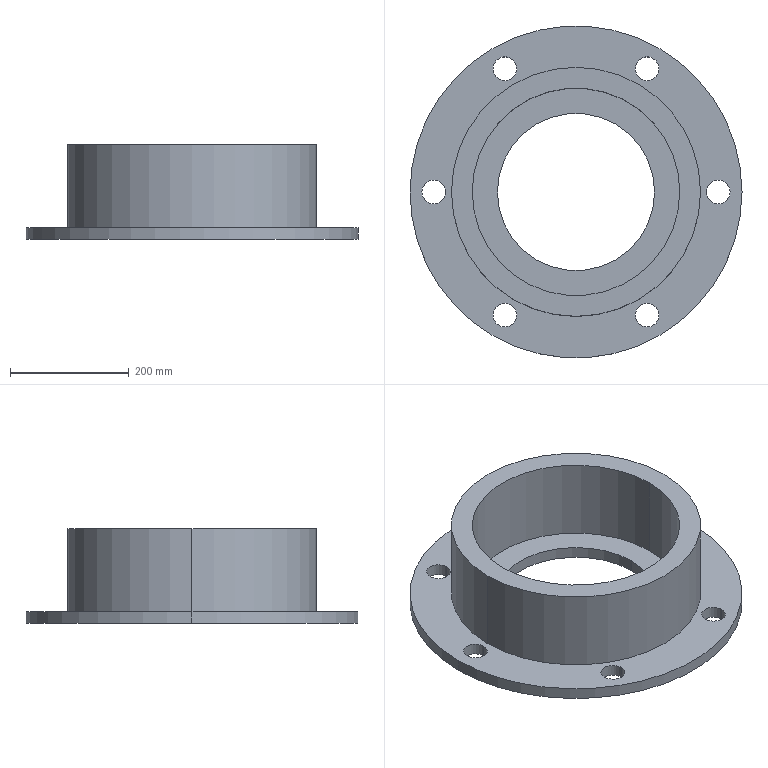Part | SolidWorks | features ICE 4, 3DProfileFeature 1, Extrusion 1 | 1 solid | 24 faces | box 560 x 560 x 160 mm | volume 9598744 mm3 | cylinder 20 | plane 4 | commonest cylinder face diameters 40 x12 265 x2 350 x2 420 x2 560 x2
STEP:
#1=CARTESIAN_POINT('',(-132.5,0.,20.));
#2=VERTEX_POINT('',#1);
#3=CARTESIAN_POINT('',(132.5,0.,20.));
#4=VERTEX_POINT('',#3);
#5=CARTESIAN_POINT('',(0.,0.,20.));
#6=DIRECTION('',(0.,0.,1.));
#7=DIRECTION('',(1.,0.,0.));
#8=AXIS2_PLACEMENT_3D('',#5,#6,#7);
#9=CIRCLE('',#8,132.5);
#10=EDGE_CURVE('',#2,#4,#9,.T.);
#11=ORIENTED_EDGE('',*,*,#10,.T.);
#12=CARTESIAN_POINT('',(132.5,0.,0.));
#13=VERTEX_POINT('',#12);
#14=CARTESIAN_POINT('',(132.5,0.,20.));
#15=DIRECTION('',(0.,0.,-1.));
#16=VECTOR('',#15,1000.);
#17=LINE('',#14,#16);
#18=EDGE_CURVE('',#4,#13,#17,.T.);
#19=ORIENTED_EDGE('',*,*,#18,.T.);
#20=CARTESIAN_POINT('',(-132.5,0.,0.));
#21=VERTEX_POINT('',#20);
#22=CARTESIAN_POINT('',(0.,0.,0.));
#23=DIRECTION('',(0.,0.,1.));
#24=DIRECTION('',(1.,0.,0.));
#25=AXIS2_PLACEMENT_3D('',#22,#23,#24);
#26=CIRCLE('',#25,132.5);
#27=EDGE_CURVE('',#21,#13,#26,.T.);
#28=ORIENTED_EDGE('',*,*,#27,.F.);
#29=CARTESIAN_POINT('',(-132.5,0.,20.));
#30=DIRECTION('',(0.,0.,-1.));
#31=VECTOR('',#30,1000.);
#32=LINE('',#29,#31);
#33=EDGE_CURVE('',#2,#21,#32,.T.);
#34=ORIENTED_EDGE('',*,*,#33,.F.);
#35=EDGE_LOOP('',(#11,#19,#28,#34));
#36=FACE_OUTER_BOUND('',#35,.T.);
#37=CARTESIAN_POINT('',(0.,0.,20.));
#38=DIRECTION('',(0.,0.,-1.));
#39=DIRECTION('',(-1.,0.,0.));
#40=AXIS2_PLACEMENT_3D('',#37,#38,#39);
#41=CYLINDRICAL_SURFACE('',#40,132.5);
#42=ADVANCED_FACE('',(#36),#41,.F.);
#43=CARTESIAN_POINT('',(220.,0.,20.));
#44=VERTEX_POINT('',#43);
#45=CARTESIAN_POINT('',(260.,0.,20.));
#46=VERTEX_POINT('',#45);
#47=CARTESIAN_POINT('',(240.,0.,20.));
#48=DIRECTION('',(0.,0.,1.));
#49=DIRECTION('',(1.,0.,0.));
#50=AXIS2_PLACEMENT_3D('',#47,#48,#49);
#51=CIRCLE('',#50,20.);
#52=EDGE_CURVE('',#44,#46,#51,.T.);
#53=ORIENTED_EDGE('',*,*,#52,.T.);
#54=CARTESIAN_POINT('',(260.,0.,0.));
#55=VERTEX_POINT('',#54);
#56=CARTESIAN_POINT('',(260.,0.,20.));
#57=DIRECTION('',(0.,0.,-1.));
#58=VECTOR('',#57,1000.);
#59=LINE('',#56,#58);
#60=EDGE_CURVE('',#46,#55,#59,.T.);
#61=ORIENTED_EDGE('',*,*,#60,.T.);
#62=CARTESIAN_POINT('',(220.,0.,0.));
#63=VERTEX_POINT('',#62);
#64=CARTESIAN_POINT('',(240.,0.,0.));
#65=DIRECTION('',(0.,0.,1.));
#66=DIRECTION('',(1.,0.,0.));
#67=AXIS2_PLACEMENT_3D('',#64,#65,#66);
#68=CIRCLE('',#67,20.);
#69=EDGE_CURVE('',#63,#55,#68,.T.);
#70=ORIENTED_EDGE('',*,*,#69,.F.);
#71=CARTESIAN_POINT('',(220.,0.,20.));
#72=DIRECTION('',(0.,0.,-1.));
#73=VECTOR('',#72,1000.);
#74=LINE('',#71,#73);
#75=EDGE_CURVE('',#44,#63,#74,.T.);
#76=ORIENTED_EDGE('',*,*,#75,.F.);
#77=EDGE_LOOP('',(#53,#61,#70,#76));
#78=FACE_OUTER_BOUND('',#77,.T.);
#79=CARTESIAN_POINT('',(240.,0.,20.));
#80=DIRECTION('',(0.,0.,-1.));
#81=DIRECTION('',(-1.,0.,0.));
#82=AXIS2_PLACEMENT_3D('',#79,#80,#81);
#83=CYLINDRICAL_SURFACE('',#82,20.);
#84=ADVANCED_FACE('',(#78),#83,.F.);
#85=CARTESIAN_POINT('',(100.,-207.846,20.));
#86=VERTEX_POINT('',#85);
#87=CARTESIAN_POINT('',(140.,-207.846,20.));
#88=VERTEX_POINT('',#87);
#89=CARTESIAN_POINT('',(120.,-207.846,20.));
#90=DIRECTION('',(0.,0.,1.));
#91=DIRECTION('',(1.,0.,0.));
#92=AXIS2_PLACEMENT_3D('',#89,#90,#91);
#93=CIRCLE('',#92,20.);
#94=EDGE_CURVE('',#86,#88,#93,.T.);
#95=ORIENTED_EDGE('',*,*,#94,.T.);
#96=CARTESIAN_POINT('',(140.,-207.846,0.));
#97=VERTEX_POINT('',#96);
#98=CARTESIAN_POINT('',(140.,-207.846,20.));
#99=DIRECTION('',(0.,0.,-1.));
#100=VECTOR('',#99,1000.);
#101=LINE('',#98,#100);
#102=EDGE_CURVE('',#88,#97,#101,.T.);
#103=ORIENTED_EDGE('',*,*,#102,.T.);
#104=CARTESIAN_POINT('',(100.,-207.846,0.));
#105=VERTEX_POINT('',#104);
#106=CARTESIAN_POINT('',(120.,-207.846,0.));
#107=DIRECTION('',(0.,0.,1.));
#108=DIRECTION('',(1.,0.,0.));
#109=AXIS2_PLACEMENT_3D('',#106,#107,#108);
#110=CIRCLE('',#109,20.);
#111=EDGE_CURVE('',#105,#97,#110,.T.);
#112=ORIENTED_EDGE('',*,*,#111,.F.);
#113=CARTESIAN_POINT('',(100.,-207.846,20.));
#114=DIRECTION('',(0.,0.,-1.));
#115=VECTOR('',#114,1000.);
#116=LINE('',#113,#115);
#117=EDGE_CURVE('',#86,#105,#116,.T.);
#118=ORIENTED_EDGE('',*,*,#117,.F.);
#119=EDGE_LOOP('',(#95,#103,#112,#118));
#120=FACE_OUTER_BOUND('',#119,.T.);
#121=CARTESIAN_POINT('',(120.,-207.846,20.));
#122=DIRECTION('',(0.,0.,-1.));
#123=DIRECTION('',(-1.,0.,0.));
#124=AXIS2_PLACEMENT_3D('',#121,#122,#123);
#125=CYLINDRICAL_SURFACE('',#124,20.);
#126=ADVANCED_FACE('',(#120),#125,.F.);
#127=CARTESIAN_POINT('',(-260.,0.,20.));
#128=VERTEX_POINT('',#127);
#129=CARTESIAN_POINT('',(-220.,0.,20.));
#130=VERTEX_POINT('',#129);
#131=CARTESIAN_POINT('',(-240.,0.,20.));
#132=DIRECTION('',(0.,0.,1.));
#133=DIRECTION('',(1.,0.,0.));
#134=AXIS2_PLACEMENT_3D('',#131,#132,#133);
#135=CIRCLE('',#134,20.);
#136=EDGE_CURVE('',#128,#130,#135,.T.);
#137=ORIENTED_EDGE('',*,*,#136,.T.);
#138=CARTESIAN_POINT('',(-220.,0.,0.));
#139=VERTEX_POINT('',#138);
#140=CARTESIAN_POINT('',(-220.,0.,20.));
#141=DIRECTION('',(0.,0.,-1.));
#142=VECTOR('',#141,1000.);
#143=LINE('',#140,#142);
#144=EDGE_CURVE('',#130,#139,#143,.T.);
#145=ORIENTED_EDGE('',*,*,#144,.T.);
#146=CARTESIAN_POINT('',(-260.,0.,0.));
#147=VERTEX_POINT('',#146);
#148=CARTESIAN_POINT('',(-240.,0.,0.));
#149=DIRECTION('',(0.,0.,1.));
#150=DIRECTION('',(1.,0.,0.));
#151=AXIS2_PLACEMENT_3D('',#148,#149,#150);
#152=CIRCLE('',#151,20.);
#153=EDGE_CURVE('',#147,#139,#152,.T.);
#154=ORIENTED_EDGE('',*,*,#153,.F.);
#155=CARTESIAN_POINT('',(-260.,0.,20.));
#156=DIRECTION('',(0.,0.,-1.));
#157=VECTOR('',#156,1000.);
#158=LINE('',#155,#157);
#159=EDGE_CURVE('',#128,#147,#158,.T.);
#160=ORIENTED_EDGE('',*,*,#159,.F.);
#161=EDGE_LOOP('',(#137,#145,#154,#160));
#162=FACE_OUTER_BOUND('',#161,.T.);
#163=CARTESIAN_POINT('',(-240.,0.,20.));
#164=DIRECTION('',(0.,0.,-1.));
#165=DIRECTION('',(-1.,0.,0.));
#166=AXIS2_PLACEMENT_3D('',#163,#164,#165);
#167=CYLINDRICAL_SURFACE('',#166,20.);
#168=ADVANCED_FACE('',(#162),#167,.F.);
#169=CARTESIAN_POINT('',(-140.,207.846,20.));
#170=VERTEX_POINT('',#169);
#171=CARTESIAN_POINT('',(-100.,207.846,20.));
#172=VERTEX_POINT('',#171);
#173=CARTESIAN_POINT('',(-120.,207.846,20.));
#174=DIRECTION('',(0.,0.,1.));
#175=DIRECTION('',(1.,0.,0.));
#176=AXIS2_PLACEMENT_3D('',#173,#174,#175);
#177=CIRCLE('',#176,20.);
#178=EDGE_CURVE('',#170,#172,#177,.T.);
#179=ORIENTED_EDGE('',*,*,#178,.T.);
#180=CARTESIAN_POINT('',(-100.,207.846,0.));
#181=VERTEX_POINT('',#180);
#182=CARTESIAN_POINT('',(-100.,207.846,20.));
#183=DIRECTION('',(0.,0.,-1.));
#184=VECTOR('',#183,1000.);
#185=LINE('',#182,#184);
#186=EDGE_CURVE('',#172,#181,#185,.T.);
#187=ORIENTED_EDGE('',*,*,#186,.T.);
#188=CARTESIAN_POINT('',(-140.,207.846,0.));
#189=VERTEX_POINT('',#188);
#190=CARTESIAN_POINT('',(-120.,207.846,0.));
#191=DIRECTION('',(0.,0.,1.));
#192=DIRECTION('',(1.,0.,0.));
#193=AXIS2_PLACEMENT_3D('',#190,#191,#192);
#194=CIRCLE('',#193,20.);
#195=EDGE_CURVE('',#189,#181,#194,.T.);
#196=ORIENTED_EDGE('',*,*,#195,.F.);
#197=CARTESIAN_POINT('',(-140.,207.846,20.));
#198=DIRECTION('',(0.,0.,-1.));
#199=VECTOR('',#198,1000.);
#200=LINE('',#197,#199);
#201=EDGE_CURVE('',#170,#189,#200,.T.);
#202=ORIENTED_EDGE('',*,*,#201,.F.);
#203=EDGE_LOOP('',(#179,#187,#196,#202));
#204=FACE_OUTER_BOUND('',#203,.T.);
#205=CARTESIAN_POINT('',(-120.,207.846,20.));
#206=DIRECTION('',(0.,0.,-1.));
#207=DIRECTION('',(-1.,0.,0.));
#208=AXIS2_PLACEMENT_3D('',#205,#206,#207);
#209=CYLINDRICAL_SURFACE('',#208,20.);
#210=ADVANCED_FACE('',(#204),#209,.F.);
#211=CARTESIAN_POINT('',(100.,207.846,20.));
#212=VERTEX_POINT('',#211);
#213=CARTESIAN_POINT('',(140.,207.846,20.));
#214=VERTEX_POINT('',#213);
#215=CARTESIAN_POINT('',(120.,207.846,20.));
#216=DIRECTION('',(0.,0.,1.));
#217=DIRECTION('',(1.,0.,0.));
#218=AXIS2_PLACEMENT_3D('',#215,#216,#217);
#219=CIRCLE('',#218,20.);
#220=EDGE_CURVE('',#212,#214,#219,.T.);
#221=ORIENTED_EDGE('',*,*,#220,.T.);
#222=CARTESIAN_POINT('',(140.,207.846,0.));
#223=VERTEX_POINT('',#222);
#224=CARTESIAN_POINT('',(140.,207.846,20.));
#225=DIRECTION('',(0.,0.,-1.));
#226=VECTOR('',#225,1000.);
#227=LINE('',#224,#226);
#228=EDGE_CURVE('',#214,#223,#227,.T.);
#229=ORIENTED_EDGE('',*,*,#228,.T.);
#230=CARTESIAN_POINT('',(100.,207.846,0.));
#231=VERTEX_POINT('',#230);
#232=CARTESIAN_POINT('',(120.,207.846,0.));
#233=DIRECTION('',(0.,0.,1.));
#234=DIRECTION('',(1.,0.,0.));
#235=AXIS2_PLACEMENT_3D('',#232,#233,#234);
#236=CIRCLE('',#235,20.);
#237=EDGE_CURVE('',#231,#223,#236,.T.);
#238=ORIENTED_EDGE('',*,*,#237,.F.);
#239=CARTESIAN_POINT('',(100.,207.846,20.));
#240=DIRECTION('',(0.,0.,-1.));
#241=VECTOR('',#240,1000.);
#242=LINE('',#239,#241);
#243=EDGE_CURVE('',#212,#231,#242,.T.);
#244=ORIENTED_EDGE('',*,*,#243,.F.);
#245=EDGE_LOOP('',(#221,#229,#238,#244));
#246=FACE_OUTER_BOUND('',#245,.T.);
#247=CARTESIAN_POINT('',(120.,207.846,20.));
#248=DIRECTION('',(0.,0.,-1.));
#249=DIRECTION('',(-1.,0.,0.));
#250=AXIS2_PLACEMENT_3D('',#247,#248,#249);
#251=CYLINDRICAL_SURFACE('',#250,20.);
#252=ADVANCED_FACE('',(#246),#251,.F.);
#253=CARTESIAN_POINT('',(-140.,-207.846,20.));
#254=VERTEX_POINT('',#253);
#255=CARTESIAN_POINT('',(-100.,-207.846,20.));
#256=VERTEX_POINT('',#255);
#257=CARTESIAN_POINT('',(-120.,-207.846,20.));
#258=DIRECTION('',(0.,0.,1.));
#259=DIRECTION('',(1.,0.,0.));
#260=AXIS2_PLACEMENT_3D('',#257,#258,#259);
#261=CIRCLE('',#260,20.);
#262=EDGE_CURVE('',#254,#256,#261,.T.);
#263=ORIENTED_EDGE('',*,*,#262,.T.);
#264=CARTESIAN_POINT('',(-100.,-207.846,0.));
#265=VERTEX_POINT('',#264);
#266=CARTESIAN_POINT('',(-100.,-207.846,20.));
#267=DIRECTION('',(0.,0.,-1.));
#268=VECTOR('',#267,1000.);
#269=LINE('',#266,#268);
#270=EDGE_CURVE('',#256,#265,#269,.T.);
#271=ORIENTED_EDGE('',*,*,#270,.T.);
#272=CARTESIAN_POINT('',(-140.,-207.846,0.));
#273=VERTEX_POINT('',#272);
#274=CARTESIAN_POINT('',(-120.,-207.846,0.));
#275=DIRECTION('',(0.,0.,1.));
#276=DIRECTION('',(1.,0.,0.));
#277=AXIS2_PLACEMENT_3D('',#274,#275,#276);
#278=CIRCLE('',#277,20.);
#279=EDGE_CURVE('',#273,#265,#278,.T.);
#280=ORIENTED_EDGE('',*,*,#279,.F.);
#281=CARTESIAN_POINT('',(-140.,-207.846,20.));
#282=DIRECTION('',(0.,0.,-1.));
#283=VECTOR('',#282,1000.);
#284=LINE('',#281,#283);
#285=EDGE_CURVE('',#254,#273,#284,.T.);
#286=ORIENTED_EDGE('',*,*,#285,.F.);
#287=EDGE_LOOP('',(#263,#271,#280,#286));
#288=FACE_OUTER_BOUND('',#287,.T.);
#289=CARTESIAN_POINT('',(-120.,-207.846,20.));
#290=DIRECTION('',(0.,0.,-1.));
#291=DIRECTION('',(-1.,0.,0.));
#292=AXIS2_PLACEMENT_3D('',#289,#290,#291);
#293=CYLINDRICAL_SURFACE('',#292,20.);
#294=ADVANCED_FACE('',(#288),#293,.F.);
#295=CARTESIAN_POINT('',(175.,0.,20.));
#296=VERTEX_POINT('',#295);
#297=CARTESIAN_POINT('',(-175.,0.,20.));
#298=VERTEX_POINT('',#297);
#299=CARTESIAN_POINT('',(0.,0.,20.));
#300=DIRECTION('',(0.,0.,-1.));
#301=DIRECTION('',(1.,0.,0.));
#302=AXIS2_PLACEMENT_3D('',#299,#300,#301);
#303=CIRCLE('',#302,175.);
#304=EDGE_CURVE('',#296,#298,#303,.T.);
#305=ORIENTED_EDGE('',*,*,#304,.T.);
#306=CARTESIAN_POINT('',(-175.,0.,160.));
#307=VERTEX_POINT('',#306);
#308=CARTESIAN_POINT('',(-175.,0.,-474.975));
#309=DIRECTION('',(0.,0.,1.));
#310=VECTOR('',#309,1000.);
#311=LINE('',#308,#310);
#312=EDGE_CURVE('',#298,#307,#311,.T.);
#313=ORIENTED_EDGE('',*,*,#312,.T.);
#314=CARTESIAN_POINT('',(175.,0.,160.));
#315=VERTEX_POINT('',#314);
#316=CARTESIAN_POINT('',(0.,0.,160.));
#317=DIRECTION('',(0.,0.,1.));
#318=DIRECTION('',(1.,0.,0.));
#319=AXIS2_PLACEMENT_3D('',#316,#317,#318);
#320=CIRCLE('',#319,175.);
#321=EDGE_CURVE('',#307,#315,#320,.T.);
#322=ORIENTED_EDGE('',*,*,#321,.T.);
#323=CARTESIAN_POINT('',(175.,0.,-474.975));
#324=DIRECTION('',(0.,0.,1.));
#325=VECTOR('',#324,1000.);
#326=LINE('',#323,#325);
#327=EDGE_CURVE('',#296,#315,#326,.T.);
#328=ORIENTED_EDGE('',*,*,#327,.F.);
#329=EDGE_LOOP('',(#305,#313,#322,#328));
#330=FACE_OUTER_BOUND('',#329,.T.);
#331=CARTESIAN_POINT('',(0.,0.,-474.975));
#332=DIRECTION('',(0.,0.,1.));
#333=DIRECTION('',(1.,0.,0.));
#334=AXIS2_PLACEMENT_3D('',#331,#332,#333);
#335=CYLINDRICAL_SURFACE('',#334,175.);
#336=ADVANCED_FACE('',(#330),#335,.F.);
#337=CARTESIAN_POINT('',(210.,0.,160.));
#338=VERTEX_POINT('',#337);
#339=CARTESIAN_POINT('',(-210.,0.,160.));
#340=VERTEX_POINT('',#339);
#341=CARTESIAN_POINT('',(0.,0.,160.));
#342=DIRECTION('',(0.,0.,1.));
#343=DIRECTION('',(1.,0.,0.));
#344=AXIS2_PLACEMENT_3D('',#341,#342,#343);
#345=CIRCLE('',#344,210.);
#346=EDGE_CURVE('',#338,#340,#345,.T.);
#347=ORIENTED_EDGE('',*,*,#346,.F.);
#348=CARTESIAN_POINT('',(210.,0.,20.));
#349=VERTEX_POINT('',#348);
#350=CARTESIAN_POINT('',(210.,0.,160.));
#351=DIRECTION('',(0.,0.,-1.));
#352=VECTOR('',#351,1000.);
#353=LINE('',#350,#352);
#354=EDGE_CURVE('',#338,#349,#353,.T.);
#355=ORIENTED_EDGE('',*,*,#354,.T.);
#356=CARTESIAN_POINT('',(-210.,0.,20.));
#357=VERTEX_POINT('',#356);
#358=CARTESIAN_POINT('',(0.,0.,20.));
#359=DIRECTION('',(0.,0.,-1.));
#360=DIRECTION('',(1.,0.,0.));
#361=AXIS2_PLACEMENT_3D('',#358,#359,#360);
#362=CIRCLE('',#361,210.);
#363=EDGE_CURVE('',#357,#349,#362,.T.);
#364=ORIENTED_EDGE('',*,*,#363,.F.);
#365=CARTESIAN_POINT('',(-210.,0.,160.));
#366=DIRECTION('',(0.,0.,-1.));
#367=VECTOR('',#366,1000.);
#368=LINE('',#365,#367);
#369=EDGE_CURVE('',#340,#357,#368,.T.);
#370=ORIENTED_EDGE('',*,*,#369,.F.);
#371=EDGE_LOOP('',(#347,#355,#364,#370));
#372=FACE_OUTER_BOUND('',#371,.T.);
#373=CARTESIAN_POINT('',(0.,0.,160.));
#374=DIRECTION('',(0.,0.,-1.));
#375=DIRECTION('',(-1.,0.,0.));
#376=AXIS2_PLACEMENT_3D('',#373,#374,#375);
#377=CYLINDRICAL_SURFACE('',#376,210.);
#378=ADVANCED_FACE('',(#372),#377,.T.);
#379=CARTESIAN_POINT('',(280.,0.,20.));
#380=VERTEX_POINT('',#379);
#381=CARTESIAN_POINT('',(-280.,0.,20.));
#382=VERTEX_POINT('',#381);
#383=CARTESIAN_POINT('',(0.,0.,20.));
#384=DIRECTION('',(0.,0.,1.));
#385=DIRECTION('',(1.,0.,0.));
#386=AXIS2_PLACEMENT_3D('',#383,#384,#385);
#387=CIRCLE('',#386,280.);
#388=EDGE_CURVE('',#380,#382,#387,.T.);
#389=ORIENTED_EDGE('',*,*,#388,.F.);
#390=CARTESIAN_POINT('',(280.,0.,0.));
#391=VERTEX_POINT('',#390);
#392=CARTESIAN_POINT('',(280.,0.,20.));
#393=DIRECTION('',(0.,0.,-1.));
#394=VECTOR('',#393,1000.);
#395=LINE('',#392,#394);
#396=EDGE_CURVE('',#380,#391,#395,.T.);
#397=ORIENTED_EDGE('',*,*,#396,.T.);
#398=CARTESIAN_POINT('',(-280.,0.,0.));
#399=VERTEX_POINT('',#398);
#400=CARTESIAN_POINT('',(0.,0.,0.));
#401=DIRECTION('',(0.,0.,1.));
#402=DIRECTION('',(1.,0.,0.));
#403=AXIS2_PLACEMENT_3D('',#400,#401,#402);
#404=CIRCLE('',#403,280.);
#405=EDGE_CURVE('',#391,#399,#404,.T.);
#406=ORIENTED_EDGE('',*,*,#405,.T.);
#407=CARTESIAN_POINT('',(-280.,0.,20.));
#408=DIRECTION('',(0.,0.,-1.));
#409=VECTOR('',#408,1000.);
#410=LINE('',#407,#409);
#411=EDGE_CURVE('',#382,#399,#410,.T.);
#412=ORIENTED_EDGE('',*,*,#411,.F.);
#413=EDGE_LOOP('',(#389,#397,#406,#412));
#414=FACE_OUTER_BOUND('',#413,.T.);
#415=CARTESIAN_POINT('',(0.,0.,20.));
#416=DIRECTION('',(0.,0.,-1.));
#417=DIRECTION('',(-1.,0.,0.));
#418=AXIS2_PLACEMENT_3D('',#415,#416,#417);
#419=CYLINDRICAL_SURFACE('',#418,280.);
#420=ADVANCED_FACE('',(#414),#419,.T.);
#421=ORIENTED_EDGE('',*,*,#396,.F.);
#422=CARTESIAN_POINT('',(0.,0.,20.));
#423=DIRECTION('',(0.,0.,1.));
#424=DIRECTION('',(1.,0.,0.));
#425=AXIS2_PLACEMENT_3D('',#422,#423,#424);
#426=CIRCLE('',#425,280.);
#427=EDGE_CURVE('',#382,#380,#426,.T.);
#428=ORIENTED_EDGE('',*,*,#427,.F.);
#429=ORIENTED_EDGE('',*,*,#411,.T.);
#430=CARTESIAN_POINT('',(0.,0.,0.));
#431=DIRECTION('',(0.,0.,1.));
#432=DIRECTION('',(1.,0.,0.));
#433=AXIS2_PLACEMENT_3D('',#430,#431,#432);
#434=CIRCLE('',#433,280.);
#435=EDGE_CURVE('',#399,#391,#434,.T.);
#436=ORIENTED_EDGE('',*,*,#435,.T.);
#437=EDGE_LOOP('',(#421,#428,#429,#436));
#438=FACE_OUTER_BOUND('',#437,.T.);
#439=CARTESIAN_POINT('',(0.,0.,20.));
#440=DIRECTION('',(0.,0.,-1.));
#441=DIRECTION('',(-1.,0.,0.));
#442=AXIS2_PLACEMENT_3D('',#439,#440,#441);
#443=CYLINDRICAL_SURFACE('',#442,280.);
#444=ADVANCED_FACE('',(#438),#443,.T.);
#445=ORIENTED_EDGE('',*,*,#52,.F.);
#446=CARTESIAN_POINT('',(240.,0.,20.));
#447=DIRECTION('',(0.,0.,1.));
#448=DIRECTION('',(1.,0.,0.));
#449=AXIS2_PLACEMENT_3D('',#446,#447,#448);
#450=CIRCLE('',#449,20.);
#451=EDGE_CURVE('',#46,#44,#450,.T.);
#452=ORIENTED_EDGE('',*,*,#451,.F.);
#453=EDGE_LOOP('',(#445,#452));
#454=FACE_BOUND('',#453,.T.);
#455=ORIENTED_EDGE('',*,*,#94,.F.);
#456=CARTESIAN_POINT('',(120.,-207.846,20.));
#457=DIRECTION('',(0.,0.,1.));
#458=DIRECTION('',(1.,0.,0.));
#459=AXIS2_PLACEMENT_3D('',#456,#457,#458);
#460=CIRCLE('',#459,20.);
#461=EDGE_CURVE('',#88,#86,#460,.T.);
#462=ORIENTED_EDGE('',*,*,#461,.F.);
#463=EDGE_LOOP('',(#455,#462));
#464=FACE_BOUND('',#463,.T.);
#465=ORIENTED_EDGE('',*,*,#136,.F.);
#466=CARTESIAN_POINT('',(-240.,0.,20.));
#467=DIRECTION('',(0.,0.,1.));
#468=DIRECTION('',(1.,0.,0.));
#469=AXIS2_PLACEMENT_3D('',#466,#467,#468);
#470=CIRCLE('',#469,20.);
#471=EDGE_CURVE('',#130,#128,#470,.T.);
#472=ORIENTED_EDGE('',*,*,#471,.F.);
#473=EDGE_LOOP('',(#465,#472));
#474=FACE_BOUND('',#473,.T.);
#475=ORIENTED_EDGE('',*,*,#178,.F.);
#476=CARTESIAN_POINT('',(-120.,207.846,20.));
#477=DIRECTION('',(0.,0.,1.));
#478=DIRECTION('',(1.,0.,0.));
#479=AXIS2_PLACEMENT_3D('',#476,#477,#478);
#480=CIRCLE('',#479,20.);
#481=EDGE_CURVE('',#172,#170,#480,.T.);
#482=ORIENTED_EDGE('',*,*,#481,.F.);
#483=EDGE_LOOP('',(#475,#482));
#484=FACE_BOUND('',#483,.T.);
#485=ORIENTED_EDGE('',*,*,#220,.F.);
#486=CARTESIAN_POINT('',(120.,207.846,20.));
#487=DIRECTION('',(0.,0.,1.));
#488=DIRECTION('',(1.,0.,0.));
#489=AXIS2_PLACEMENT_3D('',#486,#487,#488);
#490=CIRCLE('',#489,20.);
#491=EDGE_CURVE('',#214,#212,#490,.T.);
#492=ORIENTED_EDGE('',*,*,#491,.F.);
#493=EDGE_LOOP('',(#485,#492));
#494=FACE_BOUND('',#493,.T.);
#495=ORIENTED_EDGE('',*,*,#262,.F.);
#496=CARTESIAN_POINT('',(-120.,-207.846,20.));
#497=DIRECTION('',(0.,0.,1.));
#498=DIRECTION('',(1.,0.,0.));
#499=AXIS2_PLACEMENT_3D('',#496,#497,#498);
#500=CIRCLE('',#499,20.);
#501=EDGE_CURVE('',#256,#254,#500,.T.);
#502=ORIENTED_EDGE('',*,*,#501,.F.);
#503=EDGE_LOOP('',(#495,#502));
#504=FACE_BOUND('',#503,.T.);
#505=ORIENTED_EDGE('',*,*,#363,.T.);
#506=CARTESIAN_POINT('',(0.,0.,20.));
#507=DIRECTION('',(0.,0.,-1.));
#508=DIRECTION('',(1.,0.,0.));
#509=AXIS2_PLACEMENT_3D('',#506,#507,#508);
#510=CIRCLE('',#509,210.);
#511=EDGE_CURVE('',#349,#357,#510,.T.);
#512=ORIENTED_EDGE('',*,*,#511,.T.);
#513=EDGE_LOOP('',(#505,#512));
#514=FACE_BOUND('',#513,.T.);
#515=ORIENTED_EDGE('',*,*,#427,.T.);
#516=ORIENTED_EDGE('',*,*,#388,.T.);
#517=EDGE_LOOP('',(#515,#516));
#518=FACE_OUTER_BOUND('',#517,.T.);
#519=CARTESIAN_POINT('',(0.,0.,20.));
#520=DIRECTION('',(0.,0.,1.));
#521=DIRECTION('',(1.,0.,0.));
#522=AXIS2_PLACEMENT_3D('',#519,#520,#521);
#523=PLANE('',#522);
#524=ADVANCED_FACE('',(#454,#464,#474,#484,#494,#504,#514,#518),#523,.T.);
#525=ORIENTED_EDGE('',*,*,#27,.T.);
#526=CARTESIAN_POINT('',(0.,0.,0.));
#527=DIRECTION('',(0.,0.,1.));
#528=DIRECTION('',(1.,0.,0.));
#529=AXIS2_PLACEMENT_3D('',#526,#527,#528);
#530=CIRCLE('',#529,132.5);
#531=EDGE_CURVE('',#13,#21,#530,.T.);
#532=ORIENTED_EDGE('',*,*,#531,.T.);
#533=EDGE_LOOP('',(#525,#532));
#534=FACE_BOUND('',#533,.T.);
#535=ORIENTED_EDGE('',*,*,#69,.T.);
#536=CARTESIAN_POINT('',(240.,0.,0.));
#537=DIRECTION('',(0.,0.,1.));
#538=DIRECTION('',(1.,0.,0.));
#539=AXIS2_PLACEMENT_3D('',#536,#537,#538);
#540=CIRCLE('',#539,20.);
#541=EDGE_CURVE('',#55,#63,#540,.T.);
#542=ORIENTED_EDGE('',*,*,#541,.T.);
#543=EDGE_LOOP('',(#535,#542));
#544=FACE_BOUND('',#543,.T.);
#545=ORIENTED_EDGE('',*,*,#111,.T.);
#546=CARTESIAN_POINT('',(120.,-207.846,0.));
#547=DIRECTION('',(0.,0.,1.));
#548=DIRECTION('',(1.,0.,0.));
#549=AXIS2_PLACEMENT_3D('',#546,#547,#548);
#550=CIRCLE('',#549,20.);
#551=EDGE_CURVE('',#97,#105,#550,.T.);
#552=ORIENTED_EDGE('',*,*,#551,.T.);
#553=EDGE_LOOP('',(#545,#552));
#554=FACE_BOUND('',#553,.T.);
#555=ORIENTED_EDGE('',*,*,#153,.T.);
#556=CARTESIAN_POINT('',(-240.,0.,0.));
#557=DIRECTION('',(0.,0.,1.));
#558=DIRECTION('',(1.,0.,0.));
#559=AXIS2_PLACEMENT_3D('',#556,#557,#558);
#560=CIRCLE('',#559,20.);
#561=EDGE_CURVE('',#139,#147,#560,.T.);
#562=ORIENTED_EDGE('',*,*,#561,.T.);
#563=EDGE_LOOP('',(#555,#562));
#564=FACE_BOUND('',#563,.T.);
#565=ORIENTED_EDGE('',*,*,#195,.T.);
#566=CARTESIAN_POINT('',(-120.,207.846,0.));
#567=DIRECTION('',(0.,0.,1.));
#568=DIRECTION('',(1.,0.,0.));
#569=AXIS2_PLACEMENT_3D('',#566,#567,#568);
#570=CIRCLE('',#569,20.);
#571=EDGE_CURVE('',#181,#189,#570,.T.);
#572=ORIENTED_EDGE('',*,*,#571,.T.);
#573=EDGE_LOOP('',(#565,#572));
#574=FACE_BOUND('',#573,.T.);
#575=ORIENTED_EDGE('',*,*,#237,.T.);
#576=CARTESIAN_POINT('',(120.,207.846,0.));
#577=DIRECTION('',(0.,0.,1.));
#578=DIRECTION('',(1.,0.,0.));
#579=AXIS2_PLACEMENT_3D('',#576,#577,#578);
#580=CIRCLE('',#579,20.);
#581=EDGE_CURVE('',#223,#231,#580,.T.);
#582=ORIENTED_EDGE('',*,*,#581,.T.);
#583=EDGE_LOOP('',(#575,#582));
#584=FACE_BOUND('',#583,.T.);
#585=ORIENTED_EDGE('',*,*,#279,.T.);
#586=CARTESIAN_POINT('',(-120.,-207.846,0.));
#587=DIRECTION('',(0.,0.,1.));
#588=DIRECTION('',(1.,0.,0.));
#589=AXIS2_PLACEMENT_3D('',#586,#587,#588);
#590=CIRCLE('',#589,20.);
#591=EDGE_CURVE('',#265,#273,#590,.T.);
#592=ORIENTED_EDGE('',*,*,#591,.T.);
#593=EDGE_LOOP('',(#585,#592));
#594=FACE_BOUND('',#593,.T.);
#595=ORIENTED_EDGE('',*,*,#435,.F.);
#596=ORIENTED_EDGE('',*,*,#405,.F.);
#597=EDGE_LOOP('',(#595,#596));
#598=FACE_OUTER_BOUND('',#597,.T.);
#599=CARTESIAN_POINT('',(0.,0.,0.));
#600=DIRECTION('',(0.,0.,1.));
#601=DIRECTION('',(1.,0.,0.));
#602=AXIS2_PLACEMENT_3D('',#599,#600,#601);
#603=PLANE('',#602);
#604=ADVANCED_FACE('',(#534,#544,#554,#564,#574,#584,#594,#598),#603,.F.);
#605=ORIENTED_EDGE('',*,*,#354,.F.);
#606=CARTESIAN_POINT('',(0.,0.,160.));
#607=DIRECTION('',(0.,0.,1.));
#608=DIRECTION('',(1.,0.,0.));
#609=AXIS2_PLACEMENT_3D('',#606,#607,#608);
#610=CIRCLE('',#609,210.);
#611=EDGE_CURVE('',#340,#338,#610,.T.);
#612=ORIENTED_EDGE('',*,*,#611,.F.);
#613=ORIENTED_EDGE('',*,*,#369,.T.);
#614=ORIENTED_EDGE('',*,*,#511,.F.);
#615=EDGE_LOOP('',(#605,#612,#613,#614));
#616=FACE_OUTER_BOUND('',#615,.T.);
#617=CARTESIAN_POINT('',(0.,0.,160.));
#618=DIRECTION('',(0.,0.,-1.));
#619=DIRECTION('',(-1.,0.,0.));
#620=AXIS2_PLACEMENT_3D('',#617,#618,#619);
#621=CYLINDRICAL_SURFACE('',#620,210.);
#622=ADVANCED_FACE('',(#616),#621,.T.);
#623=CARTESIAN_POINT('',(0.,0.,160.));
#624=DIRECTION('',(0.,0.,1.));
#625=DIRECTION('',(1.,0.,0.));
#626=AXIS2_PLACEMENT_3D('',#623,#624,#625);
#627=CIRCLE('',#626,175.);
#628=EDGE_CURVE('',#315,#307,#627,.T.);
#629=ORIENTED_EDGE('',*,*,#628,.F.);
#630=ORIENTED_EDGE('',*,*,#321,.F.);
#631=EDGE_LOOP('',(#629,#630));
#632=FACE_BOUND('',#631,.T.);
#633=ORIENTED_EDGE('',*,*,#611,.T.);
#634=ORIENTED_EDGE('',*,*,#346,.T.);
#635=EDGE_LOOP('',(#633,#634));
#636=FACE_OUTER_BOUND('',#635,.T.);
#637=CARTESIAN_POINT('',(0.,0.,160.));
#638=DIRECTION('',(0.,0.,1.));
#639=DIRECTION('',(1.,0.,0.));
#640=AXIS2_PLACEMENT_3D('',#637,#638,#639);
#641=PLANE('',#640);
#642=ADVANCED_FACE('',(#632,#636),#641,.T.);
#643=ORIENTED_EDGE('',*,*,#312,.F.);
#644=CARTESIAN_POINT('',(0.,0.,20.));
#645=DIRECTION('',(0.,0.,-1.));
#646=DIRECTION('',(1.,0.,0.));
#647=AXIS2_PLACEMENT_3D('',#644,#645,#646);
#648=CIRCLE('',#647,175.);
#649=EDGE_CURVE('',#298,#296,#648,.T.);
#650=ORIENTED_EDGE('',*,*,#649,.T.);
#651=ORIENTED_EDGE('',*,*,#327,.T.);
#652=ORIENTED_EDGE('',*,*,#628,.T.);
#653=EDGE_LOOP('',(#643,#650,#651,#652));
#654=FACE_OUTER_BOUND('',#653,.T.);
#655=CARTESIAN_POINT('',(0.,0.,-474.975));
#656=DIRECTION('',(0.,0.,1.));
#657=DIRECTION('',(1.,0.,0.));
#658=AXIS2_PLACEMENT_3D('',#655,#656,#657);
#659=CYLINDRICAL_SURFACE('',#658,175.);
#660=ADVANCED_FACE('',(#654),#659,.F.);
#661=ORIENTED_EDGE('',*,*,#10,.F.);
#662=CARTESIAN_POINT('',(0.,0.,20.));
#663=DIRECTION('',(0.,0.,1.));
#664=DIRECTION('',(1.,0.,0.));
#665=AXIS2_PLACEMENT_3D('',#662,#663,#664);
#666=CIRCLE('',#665,132.5);
#667=EDGE_CURVE('',#4,#2,#666,.T.);
#668=ORIENTED_EDGE('',*,*,#667,.F.);
#669=EDGE_LOOP('',(#661,#668));
#670=FACE_BOUND('',#669,.T.);
#671=ORIENTED_EDGE('',*,*,#304,.F.);
#672=ORIENTED_EDGE('',*,*,#649,.F.);
#673=EDGE_LOOP('',(#671,#672));
#674=FACE_OUTER_BOUND('',#673,.T.);
#675=CARTESIAN_POINT('',(0.,0.,20.));
#676=DIRECTION('',(0.,0.,1.));
#677=DIRECTION('',(1.,0.,0.));
#678=AXIS2_PLACEMENT_3D('',#675,#676,#677);
#679=PLANE('',#678);
#680=ADVANCED_FACE('',(#670,#674),#679,.T.);
#681=ORIENTED_EDGE('',*,*,#270,.F.);
#682=ORIENTED_EDGE('',*,*,#501,.T.);
#683=ORIENTED_EDGE('',*,*,#285,.T.);
#684=ORIENTED_EDGE('',*,*,#591,.F.);
#685=EDGE_LOOP('',(#681,#682,#683,#684));
#686=FACE_OUTER_BOUND('',#685,.T.);
#687=CARTESIAN_POINT('',(-120.,-207.846,20.));
#688=DIRECTION('',(0.,0.,-1.));
#689=DIRECTION('',(-1.,0.,0.));
#690=AXIS2_PLACEMENT_3D('',#687,#688,#689);
#691=CYLINDRICAL_SURFACE('',#690,20.);
#692=ADVANCED_FACE('',(#686),#691,.F.);
#693=ORIENTED_EDGE('',*,*,#228,.F.);
#694=ORIENTED_EDGE('',*,*,#491,.T.);
#695=ORIENTED_EDGE('',*,*,#243,.T.);
#696=ORIENTED_EDGE('',*,*,#581,.F.);
#697=EDGE_LOOP('',(#693,#694,#695,#696));
#698=FACE_OUTER_BOUND('',#697,.T.);
#699=CARTESIAN_POINT('',(120.,207.846,20.));
#700=DIRECTION('',(0.,0.,-1.));
#701=DIRECTION('',(-1.,0.,0.));
#702=AXIS2_PLACEMENT_3D('',#699,#700,#701);
#703=CYLINDRICAL_SURFACE('',#702,20.);
#704=ADVANCED_FACE('',(#698),#703,.F.);
#705=ORIENTED_EDGE('',*,*,#186,.F.);
#706=ORIENTED_EDGE('',*,*,#481,.T.);
#707=ORIENTED_EDGE('',*,*,#201,.T.);
#708=ORIENTED_EDGE('',*,*,#571,.F.);
#709=EDGE_LOOP('',(#705,#706,#707,#708));
#710=FACE_OUTER_BOUND('',#709,.T.);
#711=CARTESIAN_POINT('',(-120.,207.846,20.));
#712=DIRECTION('',(0.,0.,-1.));
#713=DIRECTION('',(-1.,0.,0.));
#714=AXIS2_PLACEMENT_3D('',#711,#712,#713);
#715=CYLINDRICAL_SURFACE('',#714,20.);
#716=ADVANCED_FACE('',(#710),#715,.F.);
#717=ORIENTED_EDGE('',*,*,#144,.F.);
#718=ORIENTED_EDGE('',*,*,#471,.T.);
#719=ORIENTED_EDGE('',*,*,#159,.T.);
#720=ORIENTED_EDGE('',*,*,#561,.F.);
#721=EDGE_LOOP('',(#717,#718,#719,#720));
#722=FACE_OUTER_BOUND('',#721,.T.);
#723=CARTESIAN_POINT('',(-240.,0.,20.));
#724=DIRECTION('',(0.,0.,-1.));
#725=DIRECTION('',(-1.,0.,0.));
#726=AXIS2_PLACEMENT_3D('',#723,#724,#725);
#727=CYLINDRICAL_SURFACE('',#726,20.);
#728=ADVANCED_FACE('',(#722),#727,.F.);
#729=ORIENTED_EDGE('',*,*,#102,.F.);
#730=ORIENTED_EDGE('',*,*,#461,.T.);
#731=ORIENTED_EDGE('',*,*,#117,.T.);
#732=ORIENTED_EDGE('',*,*,#551,.F.);
#733=EDGE_LOOP('',(#729,#730,#731,#732));
#734=FACE_OUTER_BOUND('',#733,.T.);
#735=CARTESIAN_POINT('',(120.,-207.846,20.));
#736=DIRECTION('',(0.,0.,-1.));
#737=DIRECTION('',(-1.,0.,0.));
#738=AXIS2_PLACEMENT_3D('',#735,#736,#737);
#739=CYLINDRICAL_SURFACE('',#738,20.);
#740=ADVANCED_FACE('',(#734),#739,.F.);
#741=ORIENTED_EDGE('',*,*,#60,.F.);
#742=ORIENTED_EDGE('',*,*,#451,.T.);
#743=ORIENTED_EDGE('',*,*,#75,.T.);
#744=ORIENTED_EDGE('',*,*,#541,.F.);
#745=EDGE_LOOP('',(#741,#742,#743,#744));
#746=FACE_OUTER_BOUND('',#745,.T.);
#747=CARTESIAN_POINT('',(240.,0.,20.));
#748=DIRECTION('',(0.,0.,-1.));
#749=DIRECTION('',(-1.,0.,0.));
#750=AXIS2_PLACEMENT_3D('',#747,#748,#749);
#751=CYLINDRICAL_SURFACE('',#750,20.);
#752=ADVANCED_FACE('',(#746),#751,.F.);
#753=ORIENTED_EDGE('',*,*,#18,.F.);
#754=ORIENTED_EDGE('',*,*,#667,.T.);
#755=ORIENTED_EDGE('',*,*,#33,.T.);
#756=ORIENTED_EDGE('',*,*,#531,.F.);
#757=EDGE_LOOP('',(#753,#754,#755,#756));
#758=FACE_OUTER_BOUND('',#757,.T.);
#759=CARTESIAN_POINT('',(0.,0.,20.));
#760=DIRECTION('',(0.,0.,-1.));
#761=DIRECTION('',(-1.,0.,0.));
#762=AXIS2_PLACEMENT_3D('',#759,#760,#761);
#763=CYLINDRICAL_SURFACE('',#762,132.5);
#764=ADVANCED_FACE('',(#758),#763,.F.);
#765=CLOSED_SHELL('',(#42,#84,#126,#168,#210,#252,#294,#336,#378,#420,#444,#524,#604,#622,#642,#660,#680,#692,#704,#716,#728,#740,#752,#764));
#766=MANIFOLD_SOLID_BREP('',#765);
#767=CARTESIAN_POINT('',(0.,0.,0.));
#768=DIRECTION('',(0.,0.,1.));
#769=DIRECTION('',(1.,0.,0.));
#770=AXIS2_PLACEMENT_3D('',#767,#768,#769);
#771=(LENGTH_UNIT()NAMED_UNIT(*)SI_UNIT(.MILLI.,.METRE.));
#772=UNCERTAINTY_MEASURE_WITH_UNIT(LENGTH_MEASURE(0.00001),#771,'','');
#773=(NAMED_UNIT(*)PLANE_ANGLE_UNIT()SI_UNIT($,.RADIAN.));
#774=(NAMED_UNIT(*)SI_UNIT($,.STERADIAN.)SOLID_ANGLE_UNIT());
#775=(GEOMETRIC_REPRESENTATION_CONTEXT(3)GLOBAL_UNCERTAINTY_ASSIGNED_CONTEXT((#772))GLOBAL_UNIT_ASSIGNED_CONTEXT((#771,#773,#774))REPRESENTATION_CONTEXT('',''));
#776=ADVANCED_BREP_SHAPE_REPRESENTATION('',(#766,#770),#775);